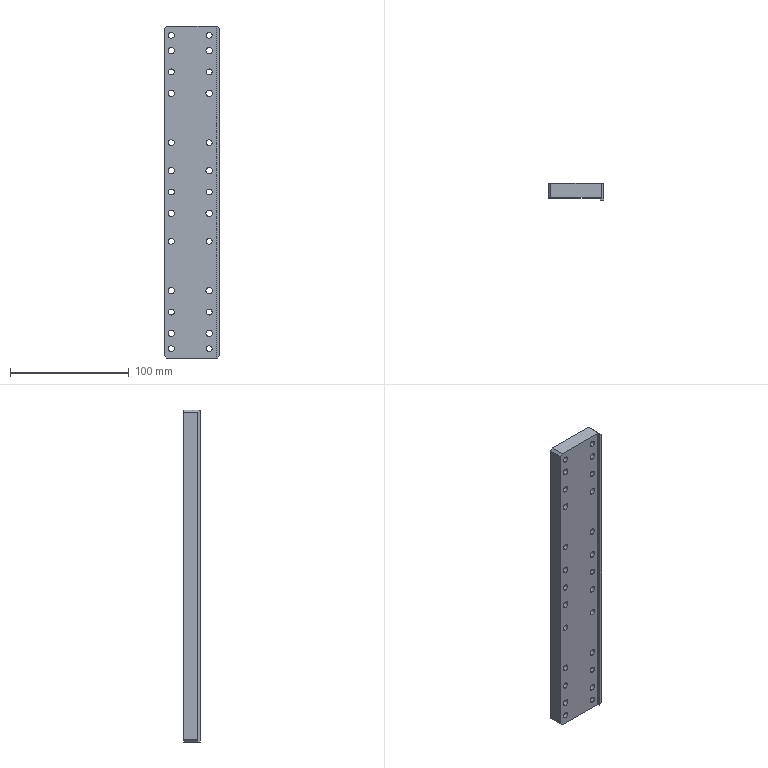Part | SolidWorks | features HoleWzd 2, Chamfer 1, Extrusion 1, MoveFace 1 | 1 solid | 100 faces | box 47 x 14 x 280 mm | volume 149226 mm3 | cylinder 76 | plane 24 | commonest cylinder face diameters 5 x28 5.5 x24 10 x24